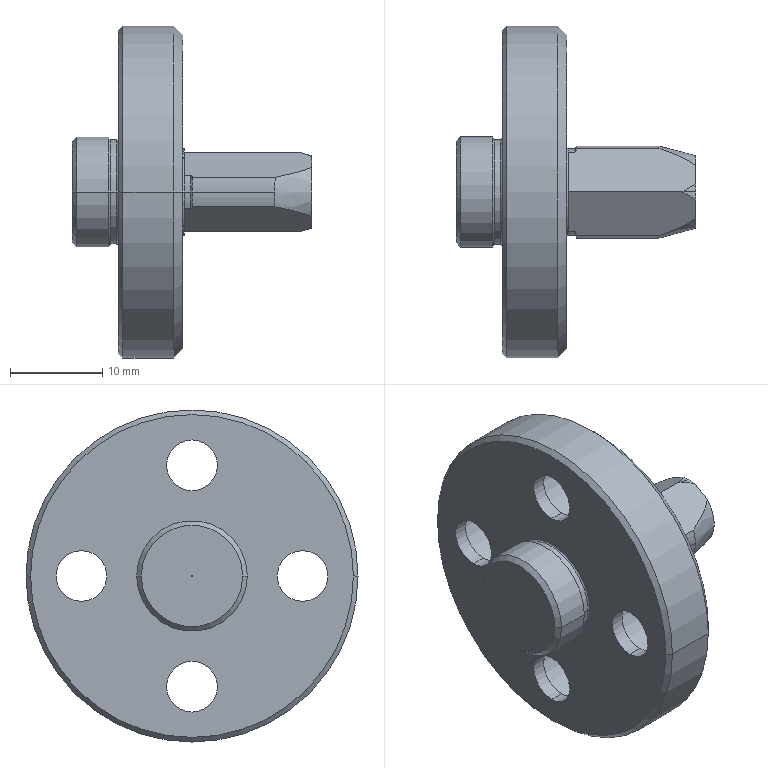Part | STEP file | MISUMI_MASDA12-P10.00-B10.0-T7.0_Locating pin | 1 solid | 69 faces | box 26 x 36 x 36 mm | volume 6690 mm3 | cylinder 28 | plane 17 | cone 15 | torus 9 | commonest cylinder face diameters 5.5 x8 9.5 x8 9.4 x3 10 x3 11.4 x2 12 x2